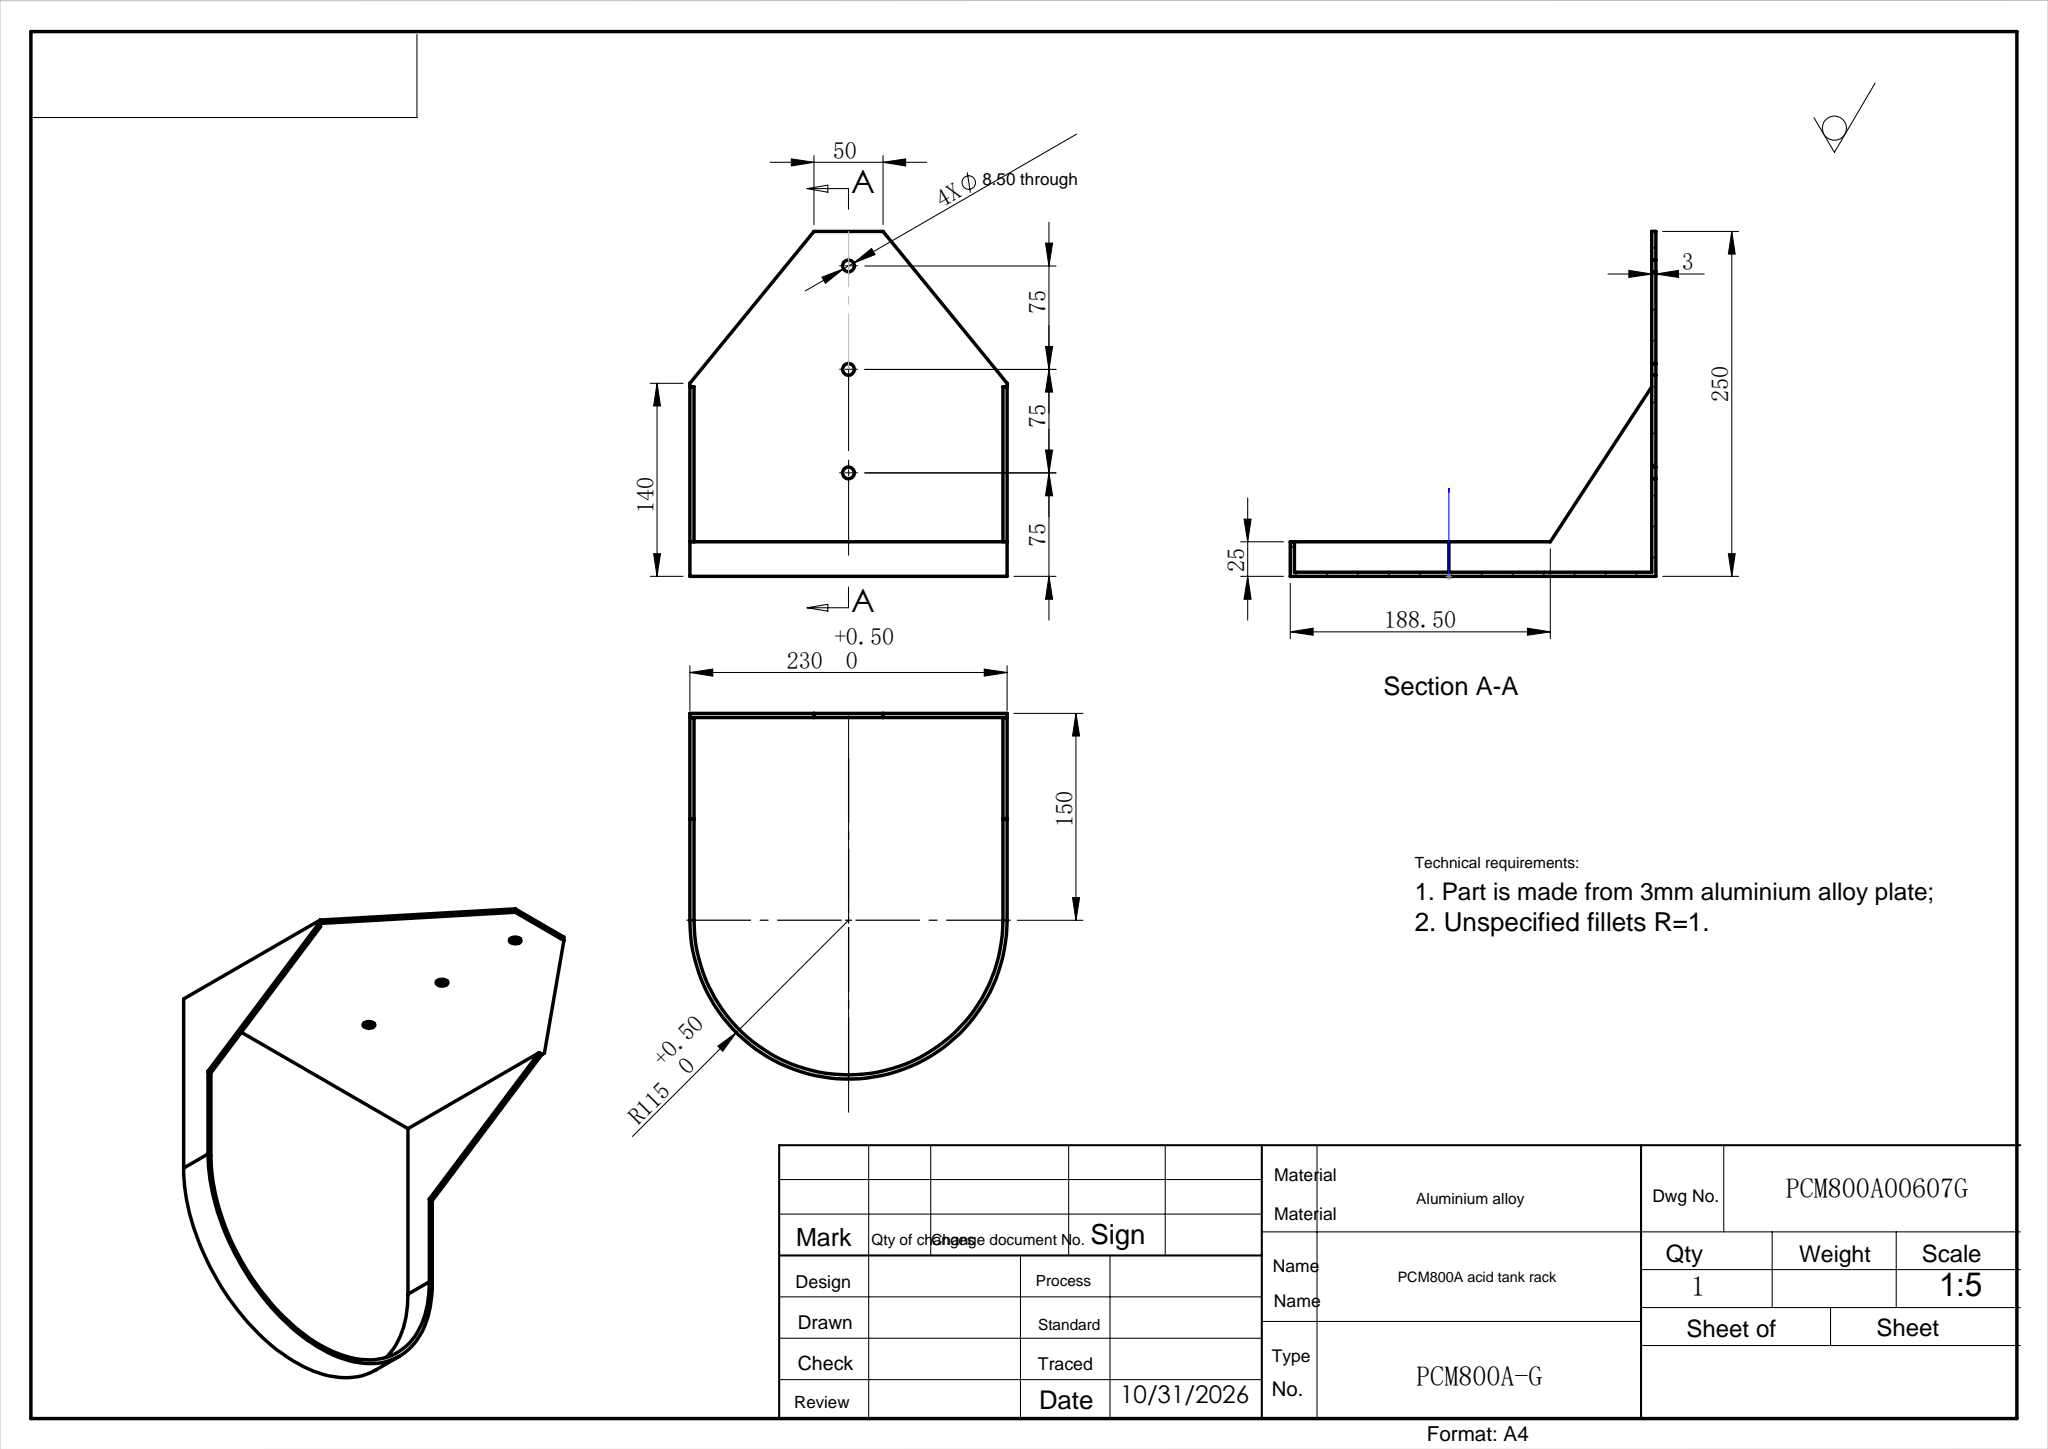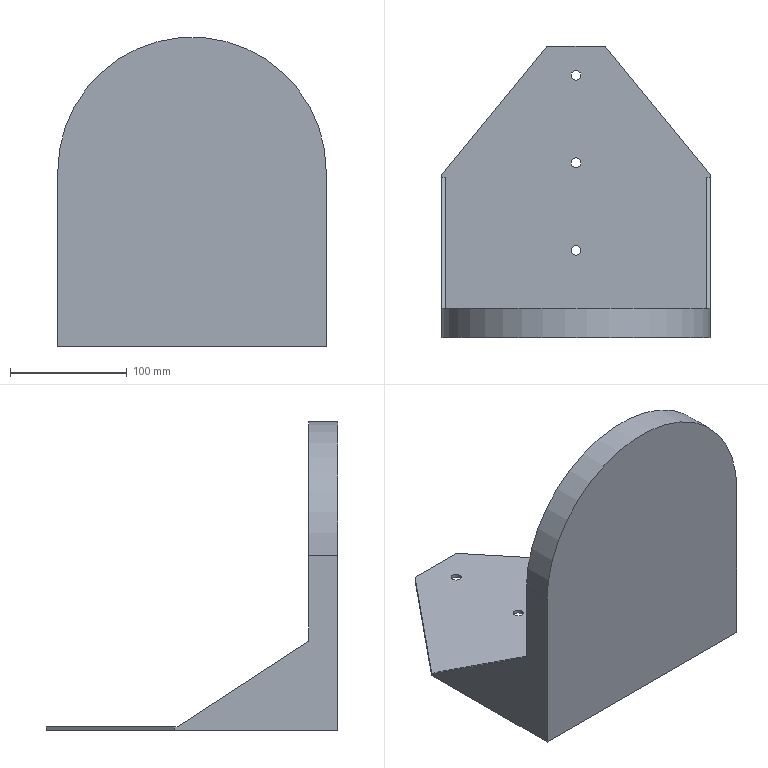Part | SolidWorks | features ICE 4, Rib 2, Extrusion 1 | 1 solid | 22 faces | box 230 x 250 x 265 mm | volume 373785 mm3 | plane 14 | cylinder 8 | commonest cylinder face diameters 8.5 x6 224 x1 230 x1
STEP:
#1=CARTESIAN_POINT('',(-4.25,75.,-147.));
#2=VERTEX_POINT('',#1);
#3=CARTESIAN_POINT('',(4.25,75.,-147.));
#4=VERTEX_POINT('',#3);
#5=CARTESIAN_POINT('',(0.,75.,-147.));
#6=DIRECTION('',(0.,0.,1.));
#7=DIRECTION('',(1.,0.,0.));
#8=AXIS2_PLACEMENT_3D('',#5,#6,#7);
#9=CIRCLE('',#8,4.25);
#10=EDGE_CURVE('',#2,#4,#9,.T.);
#11=ORIENTED_EDGE('',*,*,#10,.T.);
#12=CARTESIAN_POINT('',(4.25,75.,-150.));
#13=VERTEX_POINT('',#12);
#14=CARTESIAN_POINT('',(4.25,75.,-125.));
#15=DIRECTION('',(0.,0.,-1.));
#16=VECTOR('',#15,1000.);
#17=LINE('',#14,#16);
#18=EDGE_CURVE('',#4,#13,#17,.T.);
#19=ORIENTED_EDGE('',*,*,#18,.T.);
#20=CARTESIAN_POINT('',(-4.25,75.,-150.));
#21=VERTEX_POINT('',#20);
#22=CARTESIAN_POINT('',(0.,75.,-150.));
#23=DIRECTION('',(0.,0.,-1.));
#24=DIRECTION('',(-1.,0.,0.));
#25=AXIS2_PLACEMENT_3D('',#22,#23,#24);
#26=CIRCLE('',#25,4.25);
#27=EDGE_CURVE('',#13,#21,#26,.T.);
#28=ORIENTED_EDGE('',*,*,#27,.T.);
#29=CARTESIAN_POINT('',(-4.25,75.,-125.));
#30=DIRECTION('',(0.,0.,-1.));
#31=VECTOR('',#30,1000.);
#32=LINE('',#29,#31);
#33=EDGE_CURVE('',#2,#21,#32,.T.);
#34=ORIENTED_EDGE('',*,*,#33,.F.);
#35=EDGE_LOOP('',(#11,#19,#28,#34));
#36=FACE_OUTER_BOUND('',#35,.T.);
#37=CARTESIAN_POINT('',(0.,75.,-125.));
#38=DIRECTION('',(0.,0.,-1.));
#39=DIRECTION('',(-1.,0.,0.));
#40=AXIS2_PLACEMENT_3D('',#37,#38,#39);
#41=CYLINDRICAL_SURFACE('',#40,4.25);
#42=ADVANCED_FACE('',(#36),#41,.F.);
#43=CARTESIAN_POINT('',(-4.25,150.,-147.));
#44=VERTEX_POINT('',#43);
#45=CARTESIAN_POINT('',(4.25,150.,-147.));
#46=VERTEX_POINT('',#45);
#47=CARTESIAN_POINT('',(0.,150.,-147.));
#48=DIRECTION('',(0.,0.,1.));
#49=DIRECTION('',(1.,0.,0.));
#50=AXIS2_PLACEMENT_3D('',#47,#48,#49);
#51=CIRCLE('',#50,4.25);
#52=EDGE_CURVE('',#44,#46,#51,.T.);
#53=ORIENTED_EDGE('',*,*,#52,.T.);
#54=CARTESIAN_POINT('',(4.25,150.,-150.));
#55=VERTEX_POINT('',#54);
#56=CARTESIAN_POINT('',(4.25,150.,-125.));
#57=DIRECTION('',(0.,0.,-1.));
#58=VECTOR('',#57,1000.);
#59=LINE('',#56,#58);
#60=EDGE_CURVE('',#46,#55,#59,.T.);
#61=ORIENTED_EDGE('',*,*,#60,.T.);
#62=CARTESIAN_POINT('',(-4.25,150.,-150.));
#63=VERTEX_POINT('',#62);
#64=CARTESIAN_POINT('',(0.,150.,-150.));
#65=DIRECTION('',(0.,0.,-1.));
#66=DIRECTION('',(-1.,0.,0.));
#67=AXIS2_PLACEMENT_3D('',#64,#65,#66);
#68=CIRCLE('',#67,4.25);
#69=EDGE_CURVE('',#55,#63,#68,.T.);
#70=ORIENTED_EDGE('',*,*,#69,.T.);
#71=CARTESIAN_POINT('',(-4.25,150.,-125.));
#72=DIRECTION('',(0.,0.,-1.));
#73=VECTOR('',#72,1000.);
#74=LINE('',#71,#73);
#75=EDGE_CURVE('',#44,#63,#74,.T.);
#76=ORIENTED_EDGE('',*,*,#75,.F.);
#77=EDGE_LOOP('',(#53,#61,#70,#76));
#78=FACE_OUTER_BOUND('',#77,.T.);
#79=CARTESIAN_POINT('',(0.,150.,-125.));
#80=DIRECTION('',(0.,0.,-1.));
#81=DIRECTION('',(-1.,0.,0.));
#82=AXIS2_PLACEMENT_3D('',#79,#80,#81);
#83=CYLINDRICAL_SURFACE('',#82,4.25);
#84=ADVANCED_FACE('',(#78),#83,.F.);
#85=CARTESIAN_POINT('',(-4.25,225.,-147.));
#86=VERTEX_POINT('',#85);
#87=CARTESIAN_POINT('',(4.25,225.,-147.));
#88=VERTEX_POINT('',#87);
#89=CARTESIAN_POINT('',(0.,225.,-147.));
#90=DIRECTION('',(0.,0.,1.));
#91=DIRECTION('',(1.,0.,0.));
#92=AXIS2_PLACEMENT_3D('',#89,#90,#91);
#93=CIRCLE('',#92,4.25);
#94=EDGE_CURVE('',#86,#88,#93,.T.);
#95=ORIENTED_EDGE('',*,*,#94,.T.);
#96=CARTESIAN_POINT('',(4.25,225.,-150.));
#97=VERTEX_POINT('',#96);
#98=CARTESIAN_POINT('',(4.25,225.,-125.));
#99=DIRECTION('',(0.,0.,-1.));
#100=VECTOR('',#99,1000.);
#101=LINE('',#98,#100);
#102=EDGE_CURVE('',#88,#97,#101,.T.);
#103=ORIENTED_EDGE('',*,*,#102,.T.);
#104=CARTESIAN_POINT('',(-4.25,225.,-150.));
#105=VERTEX_POINT('',#104);
#106=CARTESIAN_POINT('',(0.,225.,-150.));
#107=DIRECTION('',(0.,0.,-1.));
#108=DIRECTION('',(-1.,0.,0.));
#109=AXIS2_PLACEMENT_3D('',#106,#107,#108);
#110=CIRCLE('',#109,4.25);
#111=EDGE_CURVE('',#97,#105,#110,.T.);
#112=ORIENTED_EDGE('',*,*,#111,.T.);
#113=CARTESIAN_POINT('',(-4.25,225.,-125.));
#114=DIRECTION('',(0.,0.,-1.));
#115=VECTOR('',#114,1000.);
#116=LINE('',#113,#115);
#117=EDGE_CURVE('',#86,#105,#116,.T.);
#118=ORIENTED_EDGE('',*,*,#117,.F.);
#119=EDGE_LOOP('',(#95,#103,#112,#118));
#120=FACE_OUTER_BOUND('',#119,.T.);
#121=CARTESIAN_POINT('',(0.,225.,-125.));
#122=DIRECTION('',(0.,0.,-1.));
#123=DIRECTION('',(-1.,0.,0.));
#124=AXIS2_PLACEMENT_3D('',#121,#122,#123);
#125=CYLINDRICAL_SURFACE('',#124,4.25);
#126=ADVANCED_FACE('',(#120),#125,.F.);
#127=CARTESIAN_POINT('',(-112.,3.,-147.));
#128=VERTEX_POINT('',#127);
#129=CARTESIAN_POINT('',(112.,3.,-147.));
#130=VERTEX_POINT('',#129);
#131=CARTESIAN_POINT('',(0.,3.,-147.));
#132=DIRECTION('',(1.,0.,0.));
#133=VECTOR('',#132,1000.);
#134=LINE('',#131,#133);
#135=EDGE_CURVE('',#128,#130,#134,.T.);
#136=ORIENTED_EDGE('',*,*,#135,.F.);
#137=CARTESIAN_POINT('',(-112.,3.,0.));
#138=VERTEX_POINT('',#137);
#139=CARTESIAN_POINT('',(-112.,3.,0.));
#140=DIRECTION('',(0.,0.,-1.));
#141=VECTOR('',#140,1000.);
#142=LINE('',#139,#141);
#143=EDGE_CURVE('',#138,#128,#142,.T.);
#144=ORIENTED_EDGE('',*,*,#143,.F.);
#145=CARTESIAN_POINT('',(112.,3.,0.));
#146=VERTEX_POINT('',#145);
#147=CARTESIAN_POINT('',(0.,3.,0.));
#148=DIRECTION('',(0.,-1.,0.));
#149=DIRECTION('',(0.,0.,1.));
#150=AXIS2_PLACEMENT_3D('',#147,#148,#149);
#151=CIRCLE('',#150,112.);
#152=EDGE_CURVE('',#146,#138,#151,.T.);
#153=ORIENTED_EDGE('',*,*,#152,.F.);
#154=CARTESIAN_POINT('',(112.,3.,0.));
#155=DIRECTION('',(0.,0.,1.));
#156=VECTOR('',#155,1000.);
#157=LINE('',#154,#156);
#158=EDGE_CURVE('',#130,#146,#157,.T.);
#159=ORIENTED_EDGE('',*,*,#158,.F.);
#160=EDGE_LOOP('',(#136,#144,#153,#159));
#161=FACE_OUTER_BOUND('',#160,.T.);
#162=CARTESIAN_POINT('',(0.,3.,0.));
#163=DIRECTION('',(0.,1.,0.));
#164=DIRECTION('',(0.,0.,1.));
#165=AXIS2_PLACEMENT_3D('',#162,#163,#164);
#166=PLANE('',#165);
#167=ADVANCED_FACE('',(#161),#166,.T.);
#168=ORIENTED_EDGE('',*,*,#10,.F.);
#169=CARTESIAN_POINT('',(0.,75.,-147.));
#170=DIRECTION('',(0.,0.,1.));
#171=DIRECTION('',(1.,0.,0.));
#172=AXIS2_PLACEMENT_3D('',#169,#170,#171);
#173=CIRCLE('',#172,4.25);
#174=EDGE_CURVE('',#4,#2,#173,.T.);
#175=ORIENTED_EDGE('',*,*,#174,.F.);
#176=EDGE_LOOP('',(#168,#175));
#177=FACE_BOUND('',#176,.T.);
#178=ORIENTED_EDGE('',*,*,#52,.F.);
#179=CARTESIAN_POINT('',(0.,150.,-147.));
#180=DIRECTION('',(0.,0.,1.));
#181=DIRECTION('',(1.,0.,0.));
#182=AXIS2_PLACEMENT_3D('',#179,#180,#181);
#183=CIRCLE('',#182,4.25);
#184=EDGE_CURVE('',#46,#44,#183,.T.);
#185=ORIENTED_EDGE('',*,*,#184,.F.);
#186=EDGE_LOOP('',(#178,#185));
#187=FACE_BOUND('',#186,.T.);
#188=ORIENTED_EDGE('',*,*,#94,.F.);
#189=CARTESIAN_POINT('',(0.,225.,-147.));
#190=DIRECTION('',(0.,0.,1.));
#191=DIRECTION('',(1.,0.,0.));
#192=AXIS2_PLACEMENT_3D('',#189,#190,#191);
#193=CIRCLE('',#192,4.25);
#194=EDGE_CURVE('',#88,#86,#193,.T.);
#195=ORIENTED_EDGE('',*,*,#194,.F.);
#196=EDGE_LOOP('',(#188,#195));
#197=FACE_BOUND('',#196,.T.);
#198=CARTESIAN_POINT('',(-115.,140.,-147.));
#199=VERTEX_POINT('',#198);
#200=CARTESIAN_POINT('',(-25.,250.,-147.));
#201=VERTEX_POINT('',#200);
#202=CARTESIAN_POINT('',(31.139,318.614,-147.));
#203=DIRECTION('',(0.6332,0.774,0.));
#204=VECTOR('',#203,1000.);
#205=LINE('',#202,#204);
#206=EDGE_CURVE('',#199,#201,#205,.T.);
#207=ORIENTED_EDGE('',*,*,#206,.F.);
#208=CARTESIAN_POINT('',(-115.,137.5,-147.));
#209=VERTEX_POINT('',#208);
#210=CARTESIAN_POINT('',(-115.,0.,-147.));
#211=DIRECTION('',(0.,1.,0.));
#212=VECTOR('',#211,1000.);
#213=LINE('',#210,#212);
#214=EDGE_CURVE('',#209,#199,#213,.T.);
#215=ORIENTED_EDGE('',*,*,#214,.F.);
#216=CARTESIAN_POINT('',(-112.,137.5,-147.));
#217=VERTEX_POINT('',#216);
#218=CARTESIAN_POINT('',(115.,137.5,-147.));
#219=DIRECTION('',(-1.,0.,0.));
#220=VECTOR('',#219,1000.);
#221=LINE('',#218,#220);
#222=EDGE_CURVE('',#217,#209,#221,.T.);
#223=ORIENTED_EDGE('',*,*,#222,.F.);
#224=CARTESIAN_POINT('',(-112.,25.,-147.));
#225=DIRECTION('',(0.,-1.,0.));
#226=VECTOR('',#225,1000.);
#227=LINE('',#224,#226);
#228=EDGE_CURVE('',#217,#128,#227,.T.);
#229=ORIENTED_EDGE('',*,*,#228,.T.);
#230=ORIENTED_EDGE('',*,*,#135,.T.);
#231=CARTESIAN_POINT('',(112.,137.5,-147.));
#232=VERTEX_POINT('',#231);
#233=CARTESIAN_POINT('',(112.,25.,-147.));
#234=DIRECTION('',(0.,-1.,0.));
#235=VECTOR('',#234,1000.);
#236=LINE('',#233,#235);
#237=EDGE_CURVE('',#232,#130,#236,.T.);
#238=ORIENTED_EDGE('',*,*,#237,.F.);
#239=CARTESIAN_POINT('',(115.,137.5,-147.));
#240=VERTEX_POINT('',#239);
#241=CARTESIAN_POINT('',(115.,137.5,-147.));
#242=DIRECTION('',(-1.,0.,0.));
#243=VECTOR('',#242,1000.);
#244=LINE('',#241,#243);
#245=EDGE_CURVE('',#240,#232,#244,.T.);
#246=ORIENTED_EDGE('',*,*,#245,.F.);
#247=CARTESIAN_POINT('',(115.,140.,-147.));
#248=VERTEX_POINT('',#247);
#249=CARTESIAN_POINT('',(115.,0.,-147.));
#250=DIRECTION('',(0.,-1.,0.));
#251=VECTOR('',#250,1000.);
#252=LINE('',#249,#251);
#253=EDGE_CURVE('',#248,#240,#252,.T.);
#254=ORIENTED_EDGE('',*,*,#253,.F.);
#255=CARTESIAN_POINT('',(25.,250.,-147.));
#256=VERTEX_POINT('',#255);
#257=CARTESIAN_POINT('',(61.089,205.891,-147.));
#258=DIRECTION('',(0.6332,-0.774,0.));
#259=VECTOR('',#258,1000.);
#260=LINE('',#257,#259);
#261=EDGE_CURVE('',#256,#248,#260,.T.);
#262=ORIENTED_EDGE('',*,*,#261,.F.);
#263=CARTESIAN_POINT('',(115.,250.,-147.));
#264=DIRECTION('',(1.,0.,0.));
#265=VECTOR('',#264,1000.);
#266=LINE('',#263,#265);
#267=EDGE_CURVE('',#201,#256,#266,.T.);
#268=ORIENTED_EDGE('',*,*,#267,.F.);
#269=EDGE_LOOP('',(#207,#215,#223,#229,#230,#238,#246,#254,#262,#268));
#270=FACE_OUTER_BOUND('',#269,.T.);
#271=CARTESIAN_POINT('',(115.,250.,-147.));
#272=DIRECTION('',(0.,0.,1.));
#273=DIRECTION('',(1.,0.,0.));
#274=AXIS2_PLACEMENT_3D('',#271,#272,#273);
#275=PLANE('',#274);
#276=ADVANCED_FACE('',(#177,#187,#197,#270),#275,.T.);
#277=CARTESIAN_POINT('',(-115.,0.,0.));
#278=VERTEX_POINT('',#277);
#279=CARTESIAN_POINT('',(115.,0.,0.));
#280=VERTEX_POINT('',#279);
#281=CARTESIAN_POINT('',(0.,0.,0.));
#282=DIRECTION('',(0.,1.,0.));
#283=DIRECTION('',(0.,0.,1.));
#284=AXIS2_PLACEMENT_3D('',#281,#282,#283);
#285=CIRCLE('',#284,115.);
#286=EDGE_CURVE('',#278,#280,#285,.T.);
#287=ORIENTED_EDGE('',*,*,#286,.T.);
#288=CARTESIAN_POINT('',(115.,25.,0.));
#289=VERTEX_POINT('',#288);
#290=CARTESIAN_POINT('',(115.,3.,0.));
#291=DIRECTION('',(0.,-1.,0.));
#292=VECTOR('',#291,1000.);
#293=LINE('',#290,#292);
#294=EDGE_CURVE('',#289,#280,#293,.T.);
#295=ORIENTED_EDGE('',*,*,#294,.F.);
#296=CARTESIAN_POINT('',(-115.,25.,0.));
#297=VERTEX_POINT('',#296);
#298=CARTESIAN_POINT('',(0.,25.,0.));
#299=DIRECTION('',(0.,1.,0.));
#300=DIRECTION('',(0.,0.,1.));
#301=AXIS2_PLACEMENT_3D('',#298,#299,#300);
#302=CIRCLE('',#301,115.);
#303=EDGE_CURVE('',#297,#289,#302,.T.);
#304=ORIENTED_EDGE('',*,*,#303,.F.);
#305=CARTESIAN_POINT('',(-115.,3.,0.));
#306=DIRECTION('',(0.,-1.,0.));
#307=VECTOR('',#306,1000.);
#308=LINE('',#305,#307);
#309=EDGE_CURVE('',#297,#278,#308,.T.);
#310=ORIENTED_EDGE('',*,*,#309,.T.);
#311=EDGE_LOOP('',(#287,#295,#304,#310));
#312=FACE_OUTER_BOUND('',#311,.T.);
#313=CARTESIAN_POINT('',(0.,3.,0.));
#314=DIRECTION('',(0.,-1.,0.));
#315=DIRECTION('',(0.,0.,-1.));
#316=AXIS2_PLACEMENT_3D('',#313,#314,#315);
#317=CYLINDRICAL_SURFACE('',#316,115.);
#318=ADVANCED_FACE('',(#312),#317,.T.);
#319=CARTESIAN_POINT('',(115.,140.,-150.));
#320=VERTEX_POINT('',#319);
#321=CARTESIAN_POINT('',(115.,0.,-150.));
#322=VERTEX_POINT('',#321);
#323=CARTESIAN_POINT('',(115.,3.,-150.));
#324=DIRECTION('',(0.,-1.,0.));
#325=VECTOR('',#324,1000.);
#326=LINE('',#323,#325);
#327=EDGE_CURVE('',#320,#322,#326,.T.);
#328=ORIENTED_EDGE('',*,*,#327,.F.);
#329=CARTESIAN_POINT('',(115.,140.,-125.));
#330=DIRECTION('',(0.,0.,-1.));
#331=VECTOR('',#330,1000.);
#332=LINE('',#329,#331);
#333=EDGE_CURVE('',#248,#320,#332,.T.);
#334=ORIENTED_EDGE('',*,*,#333,.F.);
#335=ORIENTED_EDGE('',*,*,#253,.T.);
#336=CARTESIAN_POINT('',(115.,25.,-73.5));
#337=VERTEX_POINT('',#336);
#338=CARTESIAN_POINT('',(115.,137.5,-147.));
#339=DIRECTION('',(0.,-0.8372,0.5469));
#340=VECTOR('',#339,1000.);
#341=LINE('',#338,#340);
#342=EDGE_CURVE('',#240,#337,#341,.T.);
#343=ORIENTED_EDGE('',*,*,#342,.T.);
#344=CARTESIAN_POINT('',(115.,25.,0.));
#345=DIRECTION('',(0.,0.,-1.));
#346=VECTOR('',#345,1000.);
#347=LINE('',#344,#346);
#348=EDGE_CURVE('',#289,#337,#347,.T.);
#349=ORIENTED_EDGE('',*,*,#348,.F.);
#350=ORIENTED_EDGE('',*,*,#294,.T.);
#351=CARTESIAN_POINT('',(115.,0.,0.));
#352=DIRECTION('',(0.,0.,-1.));
#353=VECTOR('',#352,1000.);
#354=LINE('',#351,#353);
#355=EDGE_CURVE('',#280,#322,#354,.T.);
#356=ORIENTED_EDGE('',*,*,#355,.T.);
#357=EDGE_LOOP('',(#328,#334,#335,#343,#349,#350,#356));
#358=FACE_OUTER_BOUND('',#357,.T.);
#359=CARTESIAN_POINT('',(115.,3.,0.));
#360=DIRECTION('',(-1.,0.,0.));
#361=DIRECTION('',(0.,0.,1.));
#362=AXIS2_PLACEMENT_3D('',#359,#360,#361);
#363=PLANE('',#362);
#364=ADVANCED_FACE('',(#358),#363,.F.);
#365=CARTESIAN_POINT('',(0.,75.,-150.));
#366=DIRECTION('',(0.,0.,-1.));
#367=DIRECTION('',(-1.,0.,0.));
#368=AXIS2_PLACEMENT_3D('',#365,#366,#367);
#369=CIRCLE('',#368,4.25);
#370=EDGE_CURVE('',#21,#13,#369,.T.);
#371=ORIENTED_EDGE('',*,*,#370,.F.);
#372=ORIENTED_EDGE('',*,*,#27,.F.);
#373=EDGE_LOOP('',(#371,#372));
#374=FACE_BOUND('',#373,.T.);
#375=CARTESIAN_POINT('',(0.,150.,-150.));
#376=DIRECTION('',(0.,0.,-1.));
#377=DIRECTION('',(-1.,0.,0.));
#378=AXIS2_PLACEMENT_3D('',#375,#376,#377);
#379=CIRCLE('',#378,4.25);
#380=EDGE_CURVE('',#63,#55,#379,.T.);
#381=ORIENTED_EDGE('',*,*,#380,.F.);
#382=ORIENTED_EDGE('',*,*,#69,.F.);
#383=EDGE_LOOP('',(#381,#382));
#384=FACE_BOUND('',#383,.T.);
#385=CARTESIAN_POINT('',(0.,225.,-150.));
#386=DIRECTION('',(0.,0.,-1.));
#387=DIRECTION('',(-1.,0.,0.));
#388=AXIS2_PLACEMENT_3D('',#385,#386,#387);
#389=CIRCLE('',#388,4.25);
#390=EDGE_CURVE('',#105,#97,#389,.T.);
#391=ORIENTED_EDGE('',*,*,#390,.F.);
#392=ORIENTED_EDGE('',*,*,#111,.F.);
#393=EDGE_LOOP('',(#391,#392));
#394=FACE_BOUND('',#393,.T.);
#395=CARTESIAN_POINT('',(-115.,140.,-150.));
#396=VERTEX_POINT('',#395);
#397=CARTESIAN_POINT('',(-115.,0.,-150.));
#398=VERTEX_POINT('',#397);
#399=CARTESIAN_POINT('',(-115.,3.,-150.));
#400=DIRECTION('',(0.,-1.,0.));
#401=VECTOR('',#400,1000.);
#402=LINE('',#399,#401);
#403=EDGE_CURVE('',#396,#398,#402,.T.);
#404=ORIENTED_EDGE('',*,*,#403,.F.);
#405=CARTESIAN_POINT('',(-25.,250.,-150.));
#406=VERTEX_POINT('',#405);
#407=CARTESIAN_POINT('',(-115.,140.,-150.));
#408=DIRECTION('',(-0.6332,-0.774,0.));
#409=VECTOR('',#408,1000.);
#410=LINE('',#407,#409);
#411=EDGE_CURVE('',#406,#396,#410,.T.);
#412=ORIENTED_EDGE('',*,*,#411,.F.);
#413=CARTESIAN_POINT('',(25.,250.,-150.));
#414=VERTEX_POINT('',#413);
#415=CARTESIAN_POINT('',(115.,250.,-150.));
#416=DIRECTION('',(1.,0.,0.));
#417=VECTOR('',#416,1000.);
#418=LINE('',#415,#417);
#419=EDGE_CURVE('',#406,#414,#418,.T.);
#420=ORIENTED_EDGE('',*,*,#419,.T.);
#421=CARTESIAN_POINT('',(115.,140.,-150.));
#422=DIRECTION('',(-0.6332,0.774,0.));
#423=VECTOR('',#422,1000.);
#424=LINE('',#421,#423);
#425=EDGE_CURVE('',#320,#414,#424,.T.);
#426=ORIENTED_EDGE('',*,*,#425,.F.);
#427=ORIENTED_EDGE('',*,*,#327,.T.);
#428=CARTESIAN_POINT('',(-115.,0.,-150.));
#429=DIRECTION('',(-1.,0.,0.));
#430=VECTOR('',#429,1000.);
#431=LINE('',#428,#430);
#432=EDGE_CURVE('',#322,#398,#431,.T.);
#433=ORIENTED_EDGE('',*,*,#432,.T.);
#434=EDGE_LOOP('',(#404,#412,#420,#426,#427,#433));
#435=FACE_OUTER_BOUND('',#434,.T.);
#436=CARTESIAN_POINT('',(-115.,3.,-150.));
#437=DIRECTION('',(0.,0.,1.));
#438=DIRECTION('',(1.,0.,0.));
#439=AXIS2_PLACEMENT_3D('',#436,#437,#438);
#440=PLANE('',#439);
#441=ADVANCED_FACE('',(#374,#384,#394,#435),#440,.F.);
#442=ORIENTED_EDGE('',*,*,#214,.T.);
#443=CARTESIAN_POINT('',(-115.,140.,-125.));
#444=DIRECTION('',(0.,0.,-1.));
#445=VECTOR('',#444,1000.);
#446=LINE('',#443,#445);
#447=EDGE_CURVE('',#199,#396,#446,.T.);
#448=ORIENTED_EDGE('',*,*,#447,.T.);
#449=ORIENTED_EDGE('',*,*,#403,.T.);
#450=CARTESIAN_POINT('',(-115.,0.,0.));
#451=DIRECTION('',(0.,0.,1.));
#452=VECTOR('',#451,1000.);
#453=LINE('',#450,#452);
#454=EDGE_CURVE('',#398,#278,#453,.T.);
#455=ORIENTED_EDGE('',*,*,#454,.T.);
#456=ORIENTED_EDGE('',*,*,#309,.F.);
#457=CARTESIAN_POINT('',(-115.,25.,-73.5));
#458=VERTEX_POINT('',#457);
#459=CARTESIAN_POINT('',(-115.,25.,0.));
#460=DIRECTION('',(0.,0.,1.));
#461=VECTOR('',#460,1000.);
#462=LINE('',#459,#461);
#463=EDGE_CURVE('',#458,#297,#462,.T.);
#464=ORIENTED_EDGE('',*,*,#463,.F.);
#465=CARTESIAN_POINT('',(-115.,137.5,-147.));
#466=DIRECTION('',(0.,-0.8372,0.5469));
#467=VECTOR('',#466,1000.);
#468=LINE('',#465,#467);
#469=EDGE_CURVE('',#209,#458,#468,.T.);
#470=ORIENTED_EDGE('',*,*,#469,.F.);
#471=EDGE_LOOP('',(#442,#448,#449,#455,#456,#464,#470));
#472=FACE_OUTER_BOUND('',#471,.T.);
#473=CARTESIAN_POINT('',(-115.,3.,0.));
#474=DIRECTION('',(1.,0.,0.));
#475=DIRECTION('',(0.,0.,-1.));
#476=AXIS2_PLACEMENT_3D('',#473,#474,#475);
#477=PLANE('',#476);
#478=ADVANCED_FACE('',(#472),#477,.F.);
#479=ORIENTED_EDGE('',*,*,#286,.F.);
#480=ORIENTED_EDGE('',*,*,#454,.F.);
#481=ORIENTED_EDGE('',*,*,#432,.F.);
#482=ORIENTED_EDGE('',*,*,#355,.F.);
#483=EDGE_LOOP('',(#479,#480,#481,#482));
#484=FACE_OUTER_BOUND('',#483,.T.);
#485=CARTESIAN_POINT('',(0.,0.,0.));
#486=DIRECTION('',(0.,1.,0.));
#487=DIRECTION('',(0.,0.,1.));
#488=AXIS2_PLACEMENT_3D('',#485,#486,#487);
#489=PLANE('',#488);
#490=ADVANCED_FACE('',(#484),#489,.F.);
#491=CARTESIAN_POINT('',(-25.,250.,-147.));
#492=DIRECTION('',(0.,0.,-1.));
#493=VECTOR('',#492,1000.);
#494=LINE('',#491,#493);
#495=EDGE_CURVE('',#201,#406,#494,.T.);
#496=ORIENTED_EDGE('',*,*,#495,.F.);
#497=ORIENTED_EDGE('',*,*,#267,.T.);
#498=CARTESIAN_POINT('',(25.,250.,-147.));
#499=DIRECTION('',(0.,0.,1.));
#500=VECTOR('',#499,1000.);
#501=LINE('',#498,#500);
#502=EDGE_CURVE('',#414,#256,#501,.T.);
#503=ORIENTED_EDGE('',*,*,#502,.F.);
#504=ORIENTED_EDGE('',*,*,#419,.F.);
#505=EDGE_LOOP('',(#496,#497,#503,#504));
#506=FACE_OUTER_BOUND('',#505,.T.);
#507=CARTESIAN_POINT('',(115.,250.,-147.));
#508=DIRECTION('',(0.,1.,0.));
#509=DIRECTION('',(0.,0.,1.));
#510=AXIS2_PLACEMENT_3D('',#507,#508,#509);
#511=PLANE('',#510);
#512=ADVANCED_FACE('',(#506),#511,.T.);
#513=ORIENTED_EDGE('',*,*,#152,.T.);
#514=CARTESIAN_POINT('',(-112.,25.,0.));
#515=VERTEX_POINT('',#514);
#516=CARTESIAN_POINT('',(-112.,25.,0.));
#517=DIRECTION('',(0.,-1.,0.));
#518=VECTOR('',#517,1000.);
#519=LINE('',#516,#518);
#520=EDGE_CURVE('',#515,#138,#519,.T.);
#521=ORIENTED_EDGE('',*,*,#520,.F.);
#522=CARTESIAN_POINT('',(112.,25.,0.));
#523=VERTEX_POINT('',#522);
#524=CARTESIAN_POINT('',(0.,25.,0.));
#525=DIRECTION('',(0.,-1.,0.));
#526=DIRECTION('',(0.,0.,1.));
#527=AXIS2_PLACEMENT_3D('',#524,#525,#526);
#528=CIRCLE('',#527,112.);
#529=EDGE_CURVE('',#523,#515,#528,.T.);
#530=ORIENTED_EDGE('',*,*,#529,.F.);
#531=CARTESIAN_POINT('',(112.,25.,0.));
#532=DIRECTION('',(0.,-1.,0.));
#533=VECTOR('',#532,1000.);
#534=LINE('',#531,#533);
#535=EDGE_CURVE('',#523,#146,#534,.T.);
#536=ORIENTED_EDGE('',*,*,#535,.T.);
#537=EDGE_LOOP('',(#513,#521,#530,#536));
#538=FACE_OUTER_BOUND('',#537,.T.);
#539=CARTESIAN_POINT('',(0.,25.,0.));
#540=DIRECTION('',(0.,-1.,0.));
#541=DIRECTION('',(0.,0.,-1.));
#542=AXIS2_PLACEMENT_3D('',#539,#540,#541);
#543=CYLINDRICAL_SURFACE('',#542,112.);
#544=ADVANCED_FACE('',(#538),#543,.F.);
#545=ORIENTED_EDGE('',*,*,#228,.F.);
#546=CARTESIAN_POINT('',(-112.,25.,-73.5));
#547=VERTEX_POINT('',#546);
#548=CARTESIAN_POINT('',(-112.,137.5,-147.));
#549=DIRECTION('',(0.,-0.8372,0.5469));
#550=VECTOR('',#549,1000.);
#551=LINE('',#548,#550);
#552=EDGE_CURVE('',#217,#547,#551,.T.);
#553=ORIENTED_EDGE('',*,*,#552,.T.);
#554=CARTESIAN_POINT('',(-112.,25.,0.));
#555=DIRECTION('',(0.,0.,-1.));
#556=VECTOR('',#555,1000.);
#557=LINE('',#554,#556);
#558=EDGE_CURVE('',#515,#547,#557,.T.);
#559=ORIENTED_EDGE('',*,*,#558,.F.);
#560=ORIENTED_EDGE('',*,*,#520,.T.);
#561=ORIENTED_EDGE('',*,*,#143,.T.);
#562=EDGE_LOOP('',(#545,#553,#559,#560,#561));
#563=FACE_OUTER_BOUND('',#562,.T.);
#564=CARTESIAN_POINT('',(-112.,25.,0.));
#565=DIRECTION('',(-1.,0.,0.));
#566=DIRECTION('',(0.,0.,1.));
#567=AXIS2_PLACEMENT_3D('',#564,#565,#566);
#568=PLANE('',#567);
#569=ADVANCED_FACE('',(#563),#568,.F.);
#570=CARTESIAN_POINT('',(112.,25.,-73.5));
#571=VERTEX_POINT('',#570);
#572=CARTESIAN_POINT('',(112.,25.,0.));
#573=DIRECTION('',(0.,0.,1.));
#574=VECTOR('',#573,1000.);
#575=LINE('',#572,#574);
#576=EDGE_CURVE('',#571,#523,#575,.T.);
#577=ORIENTED_EDGE('',*,*,#576,.F.);
#578=CARTESIAN_POINT('',(112.,137.5,-147.));
#579=DIRECTION('',(0.,-0.8372,0.5469));
#580=VECTOR('',#579,1000.);
#581=LINE('',#578,#580);
#582=EDGE_CURVE('',#232,#571,#581,.T.);
#583=ORIENTED_EDGE('',*,*,#582,.F.);
#584=ORIENTED_EDGE('',*,*,#237,.T.);
#585=ORIENTED_EDGE('',*,*,#158,.T.);
#586=ORIENTED_EDGE('',*,*,#535,.F.);
#587=EDGE_LOOP('',(#577,#583,#584,#585,#586));
#588=FACE_OUTER_BOUND('',#587,.T.);
#589=CARTESIAN_POINT('',(112.,25.,0.));
#590=DIRECTION('',(1.,0.,0.));
#591=DIRECTION('',(0.,0.,-1.));
#592=AXIS2_PLACEMENT_3D('',#589,#590,#591);
#593=PLANE('',#592);
#594=ADVANCED_FACE('',(#588),#593,.F.);
#595=CARTESIAN_POINT('',(0.,25.,-73.5));
#596=DIRECTION('',(1.,0.,0.));
#597=VECTOR('',#596,1000.);
#598=LINE('',#595,#597);
#599=EDGE_CURVE('',#458,#547,#598,.T.);
#600=ORIENTED_EDGE('',*,*,#599,.F.);
#601=ORIENTED_EDGE('',*,*,#463,.T.);
#602=ORIENTED_EDGE('',*,*,#303,.T.);
#603=ORIENTED_EDGE('',*,*,#348,.T.);
#604=CARTESIAN_POINT('',(0.,25.,-73.5));
#605=DIRECTION('',(1.,0.,0.));
#606=VECTOR('',#605,1000.);
#607=LINE('',#604,#606);
#608=EDGE_CURVE('',#571,#337,#607,.T.);
#609=ORIENTED_EDGE('',*,*,#608,.F.);
#610=ORIENTED_EDGE('',*,*,#576,.T.);
#611=ORIENTED_EDGE('',*,*,#529,.T.);
#612=ORIENTED_EDGE('',*,*,#558,.T.);
#613=EDGE_LOOP('',(#600,#601,#602,#603,#609,#610,#611,#612));
#614=FACE_OUTER_BOUND('',#613,.T.);
#615=CARTESIAN_POINT('',(0.,25.,0.));
#616=DIRECTION('',(0.,1.,0.));
#617=DIRECTION('',(0.,0.,1.));
#618=AXIS2_PLACEMENT_3D('',#615,#616,#617);
#619=PLANE('',#618);
#620=ADVANCED_FACE('',(#614),#619,.T.);
#621=ORIENTED_EDGE('',*,*,#342,.F.);
#622=ORIENTED_EDGE('',*,*,#245,.T.);
#623=ORIENTED_EDGE('',*,*,#582,.T.);
#624=ORIENTED_EDGE('',*,*,#608,.T.);
#625=EDGE_LOOP('',(#621,#622,#623,#624));
#626=FACE_OUTER_BOUND('',#625,.T.);
#627=CARTESIAN_POINT('',(115.,137.5,-147.));
#628=DIRECTION('',(0.,0.5469,0.8372));
#629=DIRECTION('',(0.,-0.8372,0.5469));
#630=AXIS2_PLACEMENT_3D('',#627,#628,#629);
#631=PLANE('',#630);
#632=ADVANCED_FACE('',(#626),#631,.T.);
#633=ORIENTED_EDGE('',*,*,#552,.F.);
#634=ORIENTED_EDGE('',*,*,#222,.T.);
#635=ORIENTED_EDGE('',*,*,#469,.T.);
#636=ORIENTED_EDGE('',*,*,#599,.T.);
#637=EDGE_LOOP('',(#633,#634,#635,#636));
#638=FACE_OUTER_BOUND('',#637,.T.);
#639=CARTESIAN_POINT('',(-115.,137.5,-147.));
#640=DIRECTION('',(0.,-0.5469,-0.8372));
#641=DIRECTION('',(0.,-0.8372,0.5469));
#642=AXIS2_PLACEMENT_3D('',#639,#640,#641);
#643=PLANE('',#642);
#644=ADVANCED_FACE('',(#638),#643,.F.);
#645=ORIENTED_EDGE('',*,*,#261,.T.);
#646=ORIENTED_EDGE('',*,*,#333,.T.);
#647=ORIENTED_EDGE('',*,*,#425,.T.);
#648=ORIENTED_EDGE('',*,*,#502,.T.);
#649=EDGE_LOOP('',(#645,#646,#647,#648));
#650=FACE_OUTER_BOUND('',#649,.T.);
#651=CARTESIAN_POINT('',(115.,140.,-125.));
#652=DIRECTION('',(-0.774,-0.6332,0.));
#653=DIRECTION('',(0.6332,-0.774,0.));
#654=AXIS2_PLACEMENT_3D('',#651,#652,#653);
#655=PLANE('',#654);
#656=ADVANCED_FACE('',(#650),#655,.F.);
#657=ORIENTED_EDGE('',*,*,#206,.T.);
#658=ORIENTED_EDGE('',*,*,#495,.T.);
#659=ORIENTED_EDGE('',*,*,#411,.T.);
#660=ORIENTED_EDGE('',*,*,#447,.F.);
#661=EDGE_LOOP('',(#657,#658,#659,#660));
#662=FACE_OUTER_BOUND('',#661,.T.);
#663=CARTESIAN_POINT('',(-115.,140.,-125.));
#664=DIRECTION('',(0.774,-0.6332,0.));
#665=DIRECTION('',(0.6332,0.774,0.));
#666=AXIS2_PLACEMENT_3D('',#663,#664,#665);
#667=PLANE('',#666);
#668=ADVANCED_FACE('',(#662),#667,.F.);
#669=ORIENTED_EDGE('',*,*,#102,.F.);
#670=ORIENTED_EDGE('',*,*,#194,.T.);
#671=ORIENTED_EDGE('',*,*,#117,.T.);
#672=ORIENTED_EDGE('',*,*,#390,.T.);
#673=EDGE_LOOP('',(#669,#670,#671,#672));
#674=FACE_OUTER_BOUND('',#673,.T.);
#675=CARTESIAN_POINT('',(0.,225.,-125.));
#676=DIRECTION('',(0.,0.,-1.));
#677=DIRECTION('',(-1.,0.,0.));
#678=AXIS2_PLACEMENT_3D('',#675,#676,#677);
#679=CYLINDRICAL_SURFACE('',#678,4.25);
#680=ADVANCED_FACE('',(#674),#679,.F.);
#681=ORIENTED_EDGE('',*,*,#60,.F.);
#682=ORIENTED_EDGE('',*,*,#184,.T.);
#683=ORIENTED_EDGE('',*,*,#75,.T.);
#684=ORIENTED_EDGE('',*,*,#380,.T.);
#685=EDGE_LOOP('',(#681,#682,#683,#684));
#686=FACE_OUTER_BOUND('',#685,.T.);
#687=CARTESIAN_POINT('',(0.,150.,-125.));
#688=DIRECTION('',(0.,0.,-1.));
#689=DIRECTION('',(-1.,0.,0.));
#690=AXIS2_PLACEMENT_3D('',#687,#688,#689);
#691=CYLINDRICAL_SURFACE('',#690,4.25);
#692=ADVANCED_FACE('',(#686),#691,.F.);
#693=ORIENTED_EDGE('',*,*,#18,.F.);
#694=ORIENTED_EDGE('',*,*,#174,.T.);
#695=ORIENTED_EDGE('',*,*,#33,.T.);
#696=ORIENTED_EDGE('',*,*,#370,.T.);
#697=EDGE_LOOP('',(#693,#694,#695,#696));
#698=FACE_OUTER_BOUND('',#697,.T.);
#699=CARTESIAN_POINT('',(0.,75.,-125.));
#700=DIRECTION('',(0.,0.,-1.));
#701=DIRECTION('',(-1.,0.,0.));
#702=AXIS2_PLACEMENT_3D('',#699,#700,#701);
#703=CYLINDRICAL_SURFACE('',#702,4.25);
#704=ADVANCED_FACE('',(#698),#703,.F.);
#705=CLOSED_SHELL('',(#42,#84,#126,#167,#276,#318,#364,#441,#478,#490,#512,#544,#569,#594,#620,#632,#644,#656,#668,#680,#692,#704));
#706=MANIFOLD_SOLID_BREP('',#705);
#707=CARTESIAN_POINT('',(0.,0.,0.));
#708=DIRECTION('',(0.,0.,1.));
#709=DIRECTION('',(1.,0.,0.));
#710=AXIS2_PLACEMENT_3D('',#707,#708,#709);
#711=(LENGTH_UNIT()NAMED_UNIT(*)SI_UNIT(.MILLI.,.METRE.));
#712=UNCERTAINTY_MEASURE_WITH_UNIT(LENGTH_MEASURE(0.00001),#711,'','');
#713=(NAMED_UNIT(*)PLANE_ANGLE_UNIT()SI_UNIT($,.RADIAN.));
#714=(NAMED_UNIT(*)SI_UNIT($,.STERADIAN.)SOLID_ANGLE_UNIT());
#715=(GEOMETRIC_REPRESENTATION_CONTEXT(3)GLOBAL_UNCERTAINTY_ASSIGNED_CONTEXT((#712))GLOBAL_UNIT_ASSIGNED_CONTEXT((#711,#713,#714))REPRESENTATION_CONTEXT('',''));
#716=ADVANCED_BREP_SHAPE_REPRESENTATION('',(#706,#710),#715);